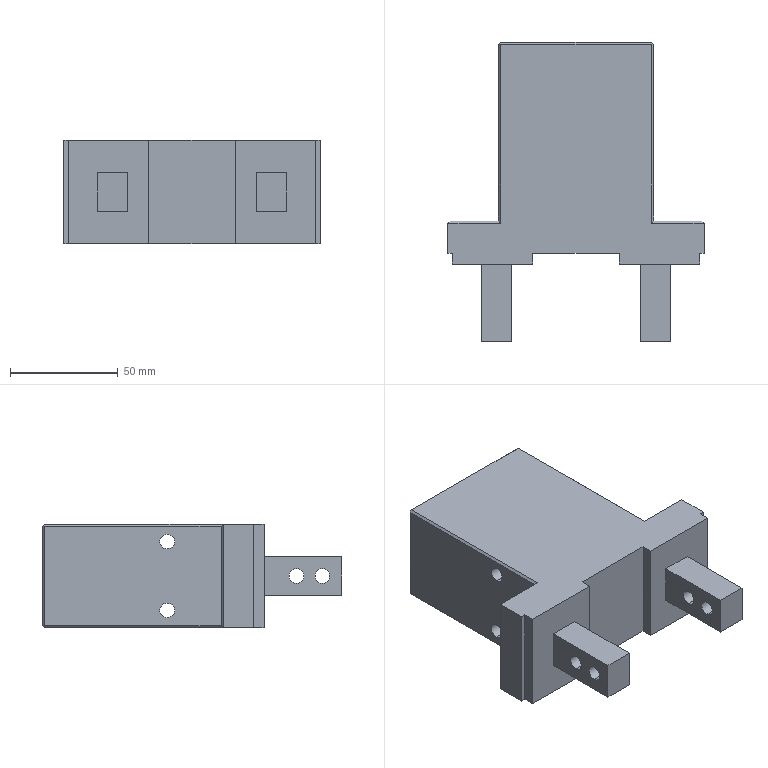Part | Creo | features DATUM PLANE 3, CURVE 2, CHAMFER 1, COORDINATE SYSTEM 1, CUT 1, PROTRUSION 1 | 1 solid | 54 faces | box 119 x 139 x 48 mm | volume 401031 mm3 | plane 42 | cylinder 12 | commonest cylinder face diameters 6.8 x12